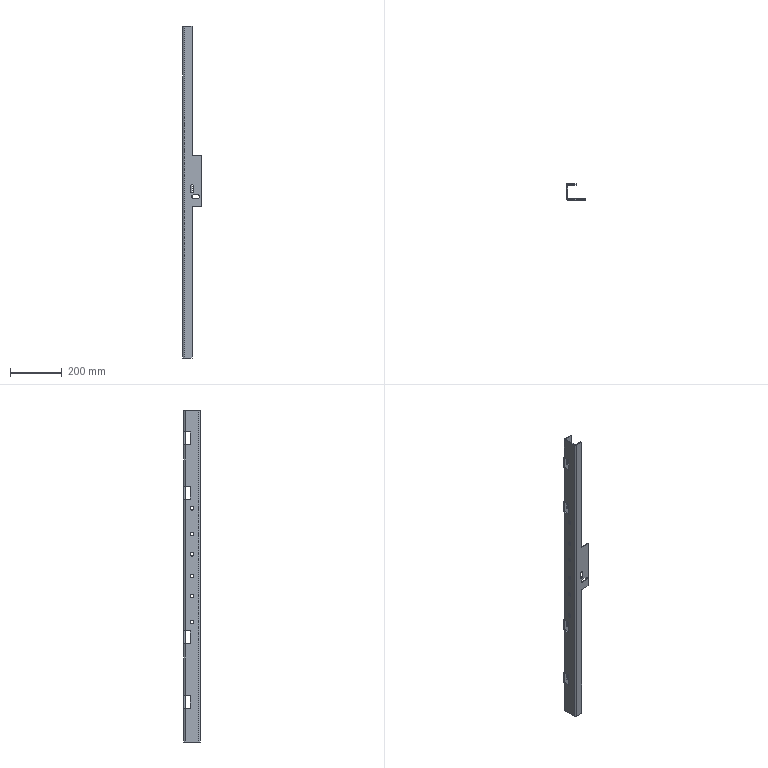Part | 1 solid | 125 faces | box 70 x 62 x 1285 mm | volume 627609 mm3 | plane 84 | cylinder 41 | commonest cylinder face diameters 14.5 x12 10 x10 0.4 x6 8.4 x6 12 x5 8 x2